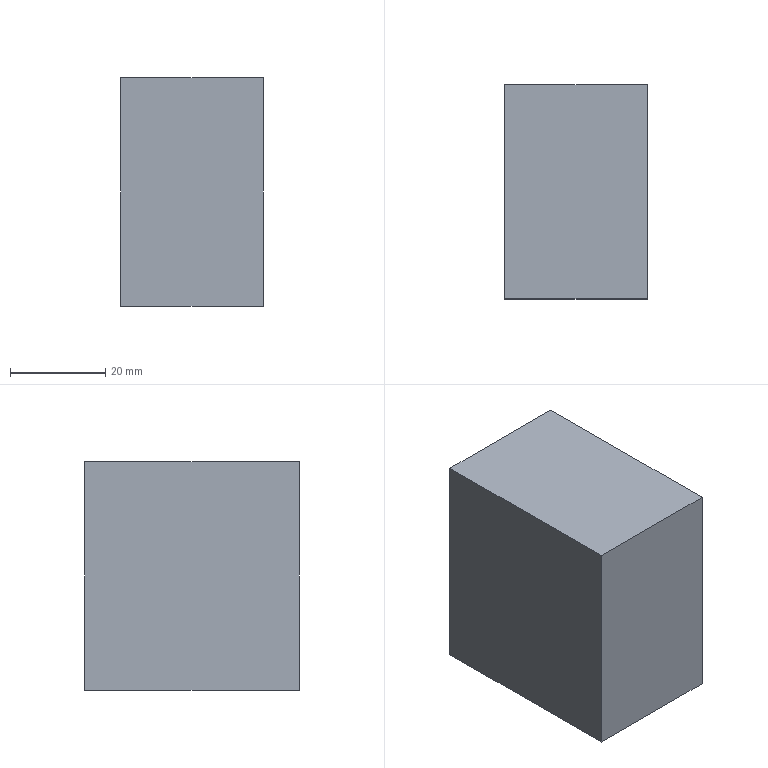Part | STEP file | 1 solid | 14 faces | box 30 x 45 x 48 mm | volume 61923 mm3 | plane 6 | cylinder 4 | cone 4 | commonest cylinder face diameters 8.5 x4
STEP:
#1=CARTESIAN_POINT('',(0.,0.,0.));
#2=DIRECTION('',(0.,0.,1.));
#3=DIRECTION('',(1.,0.,0.));
#4=AXIS2_PLACEMENT_3D('',#1,#2,#3);
#5=CARTESIAN_POINT('',(0.,20.5,-10.75));
#6=VERTEX_POINT('',#5);
#7=CARTESIAN_POINT('',(0.,45.,-10.75));
#8=VERTEX_POINT('',#7);
#9=CARTESIAN_POINT('',(0.,45.,-10.75));
#10=DIRECTION('',(0.,1.,0.));
#11=VECTOR('',#10,1.);
#12=LINE('',#9,#11);
#13=CARTESIAN_POINT('',(0.,45.,-15.));
#14=DIRECTION('',(0.,1.,0.));
#15=DIRECTION('',(0.,0.,1.));
#16=AXIS2_PLACEMENT_3D('',#13,#14,#15);
#17=CYLINDRICAL_SURFACE('',#16,4.25);
#18=CARTESIAN_POINT('',(6.283,0.));
#19=DIRECTION('',(0.,1.));
#20=VECTOR('',#19,1.);
#21=LINE('',#18,#20);
#22=(GEOMETRIC_REPRESENTATION_CONTEXT(2)PARAMETRIC_REPRESENTATION_CONTEXT()REPRESENTATION_CONTEXT('',''));
#23=DEFINITIONAL_REPRESENTATION('',(#21),#22);
#24=PCURVE('',#17,#23);
#25=CARTESIAN_POINT('',(0.,45.,-15.));
#26=DIRECTION('',(0.,1.,0.));
#27=DIRECTION('',(0.,0.,1.));
#28=AXIS2_PLACEMENT_3D('',#25,#26,#27);
#29=CYLINDRICAL_SURFACE('',#28,4.25);
#30=CARTESIAN_POINT('',(0.,0.));
#31=DIRECTION('',(0.,1.));
#32=VECTOR('',#31,1.);
#33=LINE('',#30,#32);
#34=(GEOMETRIC_REPRESENTATION_CONTEXT(2)PARAMETRIC_REPRESENTATION_CONTEXT()REPRESENTATION_CONTEXT('',''));
#35=DEFINITIONAL_REPRESENTATION('',(#33),#34);
#36=PCURVE('',#29,#35);
#37=SURFACE_CURVE('',#12,(#24,#36),.PCURVE_S1.);
#38=EDGE_CURVE('',#6,#8,#37,.T.);
#39=ORIENTED_EDGE('',*,*,#38,.T.);
#40=CARTESIAN_POINT('',(0.,45.,-19.25));
#41=VERTEX_POINT('',#40);
#42=CARTESIAN_POINT('',(0.,45.,-15.));
#43=DIRECTION('',(0.,1.,0.));
#44=DIRECTION('',(0.,0.,1.));
#45=AXIS2_PLACEMENT_3D('',#42,#43,#44);
#46=CIRCLE('',#45,4.25);
#47=CARTESIAN_POINT('',(0.,0.));
#48=DIRECTION('',(1.,0.));
#49=VECTOR('',#48,1.);
#50=LINE('',#47,#49);
#51=(GEOMETRIC_REPRESENTATION_CONTEXT(2)PARAMETRIC_REPRESENTATION_CONTEXT()REPRESENTATION_CONTEXT('',''));
#52=DEFINITIONAL_REPRESENTATION('',(#50),#51);
#53=PCURVE('',#17,#52);
#54=CARTESIAN_POINT('',(0.,45.,0.));
#55=DIRECTION('',(0.,1.,0.));
#56=DIRECTION('',(0.,0.,1.));
#57=AXIS2_PLACEMENT_3D('',#54,#55,#56);
#58=PLANE('',#57);
#59=CARTESIAN_POINT('',(-15.,0.));
#60=DIRECTION('',(1.,0.));
#61=AXIS2_PLACEMENT_2D('',#59,#60);
#62=CIRCLE('',#61,4.25);
#63=(GEOMETRIC_REPRESENTATION_CONTEXT(2)PARAMETRIC_REPRESENTATION_CONTEXT()REPRESENTATION_CONTEXT('',''));
#64=DEFINITIONAL_REPRESENTATION('',(#62),#63);
#65=PCURVE('',#58,#64);
#66=SURFACE_CURVE('',#46,(#53,#65),.PCURVE_S1.);
#67=EDGE_CURVE('',#41,#8,#66,.T.);
#68=ORIENTED_EDGE('',*,*,#67,.F.);
#69=CARTESIAN_POINT('',(0.,20.5,-19.25));
#70=VERTEX_POINT('',#69);
#71=CARTESIAN_POINT('',(0.,45.,-19.25));
#72=DIRECTION('',(0.,1.,0.));
#73=VECTOR('',#72,1.);
#74=LINE('',#71,#73);
#75=CARTESIAN_POINT('',(3.142,0.));
#76=DIRECTION('',(0.,1.));
#77=VECTOR('',#76,1.);
#78=LINE('',#75,#77);
#79=(GEOMETRIC_REPRESENTATION_CONTEXT(2)PARAMETRIC_REPRESENTATION_CONTEXT()REPRESENTATION_CONTEXT('',''));
#80=DEFINITIONAL_REPRESENTATION('',(#78),#79);
#81=PCURVE('',#17,#80);
#82=CARTESIAN_POINT('',(3.142,0.));
#83=DIRECTION('',(0.,1.));
#84=VECTOR('',#83,1.);
#85=LINE('',#82,#84);
#86=(GEOMETRIC_REPRESENTATION_CONTEXT(2)PARAMETRIC_REPRESENTATION_CONTEXT()REPRESENTATION_CONTEXT('',''));
#87=DEFINITIONAL_REPRESENTATION('',(#85),#86);
#88=PCURVE('',#29,#87);
#89=SURFACE_CURVE('',#74,(#81,#88),.PCURVE_S1.);
#90=EDGE_CURVE('',#70,#41,#89,.T.);
#91=ORIENTED_EDGE('',*,*,#90,.F.);
#92=CARTESIAN_POINT('',(0.,20.5,-15.));
#93=DIRECTION('',(0.,1.,0.));
#94=DIRECTION('',(0.,0.,1.));
#95=AXIS2_PLACEMENT_3D('',#92,#93,#94);
#96=CIRCLE('',#95,4.25);
#97=CARTESIAN_POINT('',(0.,-24.5));
#98=DIRECTION('',(1.,0.));
#99=VECTOR('',#98,1.);
#100=LINE('',#97,#99);
#101=(GEOMETRIC_REPRESENTATION_CONTEXT(2)PARAMETRIC_REPRESENTATION_CONTEXT()REPRESENTATION_CONTEXT('',''));
#102=DEFINITIONAL_REPRESENTATION('',(#100),#101);
#103=PCURVE('',#17,#102);
#104=CARTESIAN_POINT('',(0.,20.5,-15.));
#105=DIRECTION('',(0.,1.,0.));
#106=DIRECTION('',(0.,0.,1.));
#107=AXIS2_PLACEMENT_3D('',#104,#105,#106);
#108=CONICAL_SURFACE('',#107,4.25,1.03);
#109=CARTESIAN_POINT('',(0.,0.));
#110=DIRECTION('',(1.,0.));
#111=VECTOR('',#110,1.);
#112=LINE('',#109,#111);
#113=(GEOMETRIC_REPRESENTATION_CONTEXT(2)PARAMETRIC_REPRESENTATION_CONTEXT()REPRESENTATION_CONTEXT('',''));
#114=DEFINITIONAL_REPRESENTATION('',(#112),#113);
#115=PCURVE('',#108,#114);
#116=SURFACE_CURVE('',#96,(#103,#115),.PCURVE_S1.);
#117=EDGE_CURVE('',#70,#6,#116,.T.);
#118=ORIENTED_EDGE('',*,*,#117,.T.);
#119=EDGE_LOOP('',(#39,#68,#91,#118));
#120=FACE_BOUND('',#119,.F.);
#121=ADVANCED_FACE('',(#120),#17,.F.);
#122=ORIENTED_EDGE('',*,*,#117,.F.);
#123=CARTESIAN_POINT('',(0.,17.946,-15.));
#124=VERTEX_POINT('',#123);
#125=CARTESIAN_POINT('',(0.,20.5,-19.25));
#126=DIRECTION('',(0.,0.515,-0.8572));
#127=VECTOR('',#126,1.);
#128=LINE('',#125,#127);
#129=CARTESIAN_POINT('',(3.142,0.));
#130=DIRECTION('',(0.,1.));
#131=VECTOR('',#130,1.);
#132=LINE('',#129,#131);
#133=(GEOMETRIC_REPRESENTATION_CONTEXT(2)PARAMETRIC_REPRESENTATION_CONTEXT()REPRESENTATION_CONTEXT('',''));
#134=DEFINITIONAL_REPRESENTATION('',(#132),#133);
#135=PCURVE('',#108,#134);
#136=CARTESIAN_POINT('',(0.,20.5,-15.));
#137=DIRECTION('',(0.,1.,0.));
#138=DIRECTION('',(0.,0.,1.));
#139=AXIS2_PLACEMENT_3D('',#136,#137,#138);
#140=CONICAL_SURFACE('',#139,4.25,1.03);
#141=CARTESIAN_POINT('',(3.142,0.));
#142=DIRECTION('',(0.,1.));
#143=VECTOR('',#142,1.);
#144=LINE('',#141,#143);
#145=(GEOMETRIC_REPRESENTATION_CONTEXT(2)PARAMETRIC_REPRESENTATION_CONTEXT()REPRESENTATION_CONTEXT('',''));
#146=DEFINITIONAL_REPRESENTATION('',(#144),#145);
#147=PCURVE('',#140,#146);
#148=SURFACE_CURVE('',#128,(#135,#147),.PCURVE_S1.);
#149=EDGE_CURVE('',#124,#70,#148,.T.);
#150=ORIENTED_EDGE('',*,*,#149,.F.);
#151=CARTESIAN_POINT('',(0.,20.5,-10.75));
#152=DIRECTION('',(0.,0.515,0.8572));
#153=VECTOR('',#152,1.);
#154=LINE('',#151,#153);
#155=CARTESIAN_POINT('',(6.283,0.));
#156=DIRECTION('',(0.,1.));
#157=VECTOR('',#156,1.);
#158=LINE('',#155,#157);
#159=(GEOMETRIC_REPRESENTATION_CONTEXT(2)PARAMETRIC_REPRESENTATION_CONTEXT()REPRESENTATION_CONTEXT('',''));
#160=DEFINITIONAL_REPRESENTATION('',(#158),#159);
#161=PCURVE('',#108,#160);
#162=CARTESIAN_POINT('',(0.,0.));
#163=DIRECTION('',(0.,1.));
#164=VECTOR('',#163,1.);
#165=LINE('',#162,#164);
#166=(GEOMETRIC_REPRESENTATION_CONTEXT(2)PARAMETRIC_REPRESENTATION_CONTEXT()REPRESENTATION_CONTEXT('',''));
#167=DEFINITIONAL_REPRESENTATION('',(#165),#166);
#168=PCURVE('',#140,#167);
#169=SURFACE_CURVE('',#154,(#161,#168),.PCURVE_S1.);
#170=EDGE_CURVE('',#124,#6,#169,.T.);
#171=ORIENTED_EDGE('',*,*,#170,.T.);
#172=EDGE_LOOP('',(#122,#150,#171));
#173=FACE_BOUND('',#172,.F.);
#174=ADVANCED_FACE('',(#173),#108,.F.);
#175=CARTESIAN_POINT('',(0.,20.5,19.25));
#176=VERTEX_POINT('',#175);
#177=CARTESIAN_POINT('',(0.,45.,19.25));
#178=VERTEX_POINT('',#177);
#179=CARTESIAN_POINT('',(0.,45.,19.25));
#180=DIRECTION('',(0.,1.,0.));
#181=VECTOR('',#180,1.);
#182=LINE('',#179,#181);
#183=CARTESIAN_POINT('',(0.,45.,15.));
#184=DIRECTION('',(0.,1.,0.));
#185=DIRECTION('',(0.,0.,1.));
#186=AXIS2_PLACEMENT_3D('',#183,#184,#185);
#187=CYLINDRICAL_SURFACE('',#186,4.25);
#188=CARTESIAN_POINT('',(6.283,0.));
#189=DIRECTION('',(0.,1.));
#190=VECTOR('',#189,1.);
#191=LINE('',#188,#190);
#192=(GEOMETRIC_REPRESENTATION_CONTEXT(2)PARAMETRIC_REPRESENTATION_CONTEXT()REPRESENTATION_CONTEXT('',''));
#193=DEFINITIONAL_REPRESENTATION('',(#191),#192);
#194=PCURVE('',#187,#193);
#195=CARTESIAN_POINT('',(0.,45.,15.));
#196=DIRECTION('',(0.,1.,0.));
#197=DIRECTION('',(0.,0.,1.));
#198=AXIS2_PLACEMENT_3D('',#195,#196,#197);
#199=CYLINDRICAL_SURFACE('',#198,4.25);
#200=CARTESIAN_POINT('',(0.,0.));
#201=DIRECTION('',(0.,1.));
#202=VECTOR('',#201,1.);
#203=LINE('',#200,#202);
#204=(GEOMETRIC_REPRESENTATION_CONTEXT(2)PARAMETRIC_REPRESENTATION_CONTEXT()REPRESENTATION_CONTEXT('',''));
#205=DEFINITIONAL_REPRESENTATION('',(#203),#204);
#206=PCURVE('',#199,#205);
#207=SURFACE_CURVE('',#182,(#194,#206),.PCURVE_S1.);
#208=EDGE_CURVE('',#176,#178,#207,.T.);
#209=ORIENTED_EDGE('',*,*,#208,.T.);
#210=CARTESIAN_POINT('',(0.,45.,10.75));
#211=VERTEX_POINT('',#210);
#212=CARTESIAN_POINT('',(0.,45.,15.));
#213=DIRECTION('',(0.,1.,0.));
#214=DIRECTION('',(0.,0.,1.));
#215=AXIS2_PLACEMENT_3D('',#212,#213,#214);
#216=CIRCLE('',#215,4.25);
#217=CARTESIAN_POINT('',(0.,0.));
#218=DIRECTION('',(1.,0.));
#219=VECTOR('',#218,1.);
#220=LINE('',#217,#219);
#221=(GEOMETRIC_REPRESENTATION_CONTEXT(2)PARAMETRIC_REPRESENTATION_CONTEXT()REPRESENTATION_CONTEXT('',''));
#222=DEFINITIONAL_REPRESENTATION('',(#220),#221);
#223=PCURVE('',#187,#222);
#224=CARTESIAN_POINT('',(15.,0.));
#225=DIRECTION('',(1.,0.));
#226=AXIS2_PLACEMENT_2D('',#224,#225);
#227=CIRCLE('',#226,4.25);
#228=(GEOMETRIC_REPRESENTATION_CONTEXT(2)PARAMETRIC_REPRESENTATION_CONTEXT()REPRESENTATION_CONTEXT('',''));
#229=DEFINITIONAL_REPRESENTATION('',(#227),#228);
#230=PCURVE('',#58,#229);
#231=SURFACE_CURVE('',#216,(#223,#230),.PCURVE_S1.);
#232=EDGE_CURVE('',#211,#178,#231,.T.);
#233=ORIENTED_EDGE('',*,*,#232,.F.);
#234=CARTESIAN_POINT('',(0.,20.5,10.75));
#235=VERTEX_POINT('',#234);
#236=CARTESIAN_POINT('',(0.,45.,10.75));
#237=DIRECTION('',(0.,1.,0.));
#238=VECTOR('',#237,1.);
#239=LINE('',#236,#238);
#240=CARTESIAN_POINT('',(3.142,0.));
#241=DIRECTION('',(0.,1.));
#242=VECTOR('',#241,1.);
#243=LINE('',#240,#242);
#244=(GEOMETRIC_REPRESENTATION_CONTEXT(2)PARAMETRIC_REPRESENTATION_CONTEXT()REPRESENTATION_CONTEXT('',''));
#245=DEFINITIONAL_REPRESENTATION('',(#243),#244);
#246=PCURVE('',#187,#245);
#247=CARTESIAN_POINT('',(3.142,0.));
#248=DIRECTION('',(0.,1.));
#249=VECTOR('',#248,1.);
#250=LINE('',#247,#249);
#251=(GEOMETRIC_REPRESENTATION_CONTEXT(2)PARAMETRIC_REPRESENTATION_CONTEXT()REPRESENTATION_CONTEXT('',''));
#252=DEFINITIONAL_REPRESENTATION('',(#250),#251);
#253=PCURVE('',#199,#252);
#254=SURFACE_CURVE('',#239,(#246,#253),.PCURVE_S1.);
#255=EDGE_CURVE('',#235,#211,#254,.T.);
#256=ORIENTED_EDGE('',*,*,#255,.F.);
#257=CARTESIAN_POINT('',(0.,20.5,15.));
#258=DIRECTION('',(0.,1.,0.));
#259=DIRECTION('',(0.,0.,1.));
#260=AXIS2_PLACEMENT_3D('',#257,#258,#259);
#261=CIRCLE('',#260,4.25);
#262=CARTESIAN_POINT('',(0.,-24.5));
#263=DIRECTION('',(1.,0.));
#264=VECTOR('',#263,1.);
#265=LINE('',#262,#264);
#266=(GEOMETRIC_REPRESENTATION_CONTEXT(2)PARAMETRIC_REPRESENTATION_CONTEXT()REPRESENTATION_CONTEXT('',''));
#267=DEFINITIONAL_REPRESENTATION('',(#265),#266);
#268=PCURVE('',#187,#267);
#269=CARTESIAN_POINT('',(0.,20.5,15.));
#270=DIRECTION('',(0.,1.,0.));
#271=DIRECTION('',(0.,0.,1.));
#272=AXIS2_PLACEMENT_3D('',#269,#270,#271);
#273=CONICAL_SURFACE('',#272,4.25,1.03);
#274=CARTESIAN_POINT('',(0.,0.));
#275=DIRECTION('',(1.,0.));
#276=VECTOR('',#275,1.);
#277=LINE('',#274,#276);
#278=(GEOMETRIC_REPRESENTATION_CONTEXT(2)PARAMETRIC_REPRESENTATION_CONTEXT()REPRESENTATION_CONTEXT('',''));
#279=DEFINITIONAL_REPRESENTATION('',(#277),#278);
#280=PCURVE('',#273,#279);
#281=SURFACE_CURVE('',#261,(#268,#280),.PCURVE_S1.);
#282=EDGE_CURVE('',#235,#176,#281,.T.);
#283=ORIENTED_EDGE('',*,*,#282,.T.);
#284=EDGE_LOOP('',(#209,#233,#256,#283));
#285=FACE_BOUND('',#284,.F.);
#286=ADVANCED_FACE('',(#285),#187,.F.);
#287=ORIENTED_EDGE('',*,*,#282,.F.);
#288=CARTESIAN_POINT('',(0.,17.946,15.));
#289=VERTEX_POINT('',#288);
#290=CARTESIAN_POINT('',(0.,20.5,10.75));
#291=DIRECTION('',(0.,0.515,-0.8572));
#292=VECTOR('',#291,1.);
#293=LINE('',#290,#292);
#294=CARTESIAN_POINT('',(3.142,0.));
#295=DIRECTION('',(0.,1.));
#296=VECTOR('',#295,1.);
#297=LINE('',#294,#296);
#298=(GEOMETRIC_REPRESENTATION_CONTEXT(2)PARAMETRIC_REPRESENTATION_CONTEXT()REPRESENTATION_CONTEXT('',''));
#299=DEFINITIONAL_REPRESENTATION('',(#297),#298);
#300=PCURVE('',#273,#299);
#301=CARTESIAN_POINT('',(0.,20.5,15.));
#302=DIRECTION('',(0.,1.,0.));
#303=DIRECTION('',(0.,0.,1.));
#304=AXIS2_PLACEMENT_3D('',#301,#302,#303);
#305=CONICAL_SURFACE('',#304,4.25,1.03);
#306=CARTESIAN_POINT('',(3.142,0.));
#307=DIRECTION('',(0.,1.));
#308=VECTOR('',#307,1.);
#309=LINE('',#306,#308);
#310=(GEOMETRIC_REPRESENTATION_CONTEXT(2)PARAMETRIC_REPRESENTATION_CONTEXT()REPRESENTATION_CONTEXT('',''));
#311=DEFINITIONAL_REPRESENTATION('',(#309),#310);
#312=PCURVE('',#305,#311);
#313=SURFACE_CURVE('',#293,(#300,#312),.PCURVE_S1.);
#314=EDGE_CURVE('',#289,#235,#313,.T.);
#315=ORIENTED_EDGE('',*,*,#314,.F.);
#316=CARTESIAN_POINT('',(0.,20.5,19.25));
#317=DIRECTION('',(0.,0.515,0.8572));
#318=VECTOR('',#317,1.);
#319=LINE('',#316,#318);
#320=CARTESIAN_POINT('',(6.283,0.));
#321=DIRECTION('',(0.,1.));
#322=VECTOR('',#321,1.);
#323=LINE('',#320,#322);
#324=(GEOMETRIC_REPRESENTATION_CONTEXT(2)PARAMETRIC_REPRESENTATION_CONTEXT()REPRESENTATION_CONTEXT('',''));
#325=DEFINITIONAL_REPRESENTATION('',(#323),#324);
#326=PCURVE('',#273,#325);
#327=CARTESIAN_POINT('',(0.,0.));
#328=DIRECTION('',(0.,1.));
#329=VECTOR('',#328,1.);
#330=LINE('',#327,#329);
#331=(GEOMETRIC_REPRESENTATION_CONTEXT(2)PARAMETRIC_REPRESENTATION_CONTEXT()REPRESENTATION_CONTEXT('',''));
#332=DEFINITIONAL_REPRESENTATION('',(#330),#331);
#333=PCURVE('',#305,#332);
#334=SURFACE_CURVE('',#319,(#326,#333),.PCURVE_S1.);
#335=EDGE_CURVE('',#289,#176,#334,.T.);
#336=ORIENTED_EDGE('',*,*,#335,.T.);
#337=EDGE_LOOP('',(#287,#315,#336));
#338=FACE_BOUND('',#337,.F.);
#339=ADVANCED_FACE('',(#338),#273,.F.);
#340=CARTESIAN_POINT('',(-15.,0.,-24.));
#341=VERTEX_POINT('',#340);
#342=CARTESIAN_POINT('',(-15.,0.,24.));
#343=VERTEX_POINT('',#342);
#344=CARTESIAN_POINT('',(-15.,0.,24.));
#345=DIRECTION('',(0.,0.,1.));
#346=VECTOR('',#345,1.);
#347=LINE('',#344,#346);
#348=CARTESIAN_POINT('',(-15.,45.,24.));
#349=DIRECTION('',(1.,0.,0.));
#350=DIRECTION('',(0.,0.,-1.));
#351=AXIS2_PLACEMENT_3D('',#348,#349,#350);
#352=PLANE('',#351);
#353=CARTESIAN_POINT('',(0.,-45.));
#354=DIRECTION('',(-1.,0.));
#355=VECTOR('',#354,1.);
#356=LINE('',#353,#355);
#357=(GEOMETRIC_REPRESENTATION_CONTEXT(2)PARAMETRIC_REPRESENTATION_CONTEXT()REPRESENTATION_CONTEXT('',''));
#358=DEFINITIONAL_REPRESENTATION('',(#356),#357);
#359=PCURVE('',#352,#358);
#360=CARTESIAN_POINT('',(0.,0.,0.));
#361=DIRECTION('',(0.,1.,0.));
#362=DIRECTION('',(0.,0.,1.));
#363=AXIS2_PLACEMENT_3D('',#360,#361,#362);
#364=PLANE('',#363);
#365=CARTESIAN_POINT('',(24.,-15.));
#366=DIRECTION('',(1.,0.));
#367=VECTOR('',#366,1.);
#368=LINE('',#365,#367);
#369=(GEOMETRIC_REPRESENTATION_CONTEXT(2)PARAMETRIC_REPRESENTATION_CONTEXT()REPRESENTATION_CONTEXT('',''));
#370=DEFINITIONAL_REPRESENTATION('',(#368),#369);
#371=PCURVE('',#364,#370);
#372=SURFACE_CURVE('',#347,(#359,#371),.PCURVE_S1.);
#373=EDGE_CURVE('',#341,#343,#372,.T.);
#374=ORIENTED_EDGE('',*,*,#373,.T.);
#375=CARTESIAN_POINT('',(-15.,45.,24.));
#376=VERTEX_POINT('',#375);
#377=CARTESIAN_POINT('',(-15.,45.,24.));
#378=DIRECTION('',(0.,-1.,0.));
#379=VECTOR('',#378,1.);
#380=LINE('',#377,#379);
#381=CARTESIAN_POINT('',(0.,0.));
#382=DIRECTION('',(0.,-1.));
#383=VECTOR('',#382,1.);
#384=LINE('',#381,#383);
#385=(GEOMETRIC_REPRESENTATION_CONTEXT(2)PARAMETRIC_REPRESENTATION_CONTEXT()REPRESENTATION_CONTEXT('',''));
#386=DEFINITIONAL_REPRESENTATION('',(#384),#385);
#387=PCURVE('',#352,#386);
#388=CARTESIAN_POINT('',(15.,45.,24.));
#389=DIRECTION('',(0.,0.,-1.));
#390=DIRECTION('',(-1.,0.,0.));
#391=AXIS2_PLACEMENT_3D('',#388,#389,#390);
#392=PLANE('',#391);
#393=CARTESIAN_POINT('',(30.,0.));
#394=DIRECTION('',(0.,-1.));
#395=VECTOR('',#394,1.);
#396=LINE('',#393,#395);
#397=(GEOMETRIC_REPRESENTATION_CONTEXT(2)PARAMETRIC_REPRESENTATION_CONTEXT()REPRESENTATION_CONTEXT('',''));
#398=DEFINITIONAL_REPRESENTATION('',(#396),#397);
#399=PCURVE('',#392,#398);
#400=SURFACE_CURVE('',#380,(#387,#399),.PCURVE_S1.);
#401=EDGE_CURVE('',#376,#343,#400,.T.);
#402=ORIENTED_EDGE('',*,*,#401,.F.);
#403=CARTESIAN_POINT('',(-15.,45.,-24.));
#404=VERTEX_POINT('',#403);
#405=CARTESIAN_POINT('',(-15.,45.,24.));
#406=DIRECTION('',(0.,0.,1.));
#407=VECTOR('',#406,1.);
#408=LINE('',#405,#407);
#409=CARTESIAN_POINT('',(0.,0.));
#410=DIRECTION('',(-1.,0.));
#411=VECTOR('',#410,1.);
#412=LINE('',#409,#411);
#413=(GEOMETRIC_REPRESENTATION_CONTEXT(2)PARAMETRIC_REPRESENTATION_CONTEXT()REPRESENTATION_CONTEXT('',''));
#414=DEFINITIONAL_REPRESENTATION('',(#412),#413);
#415=PCURVE('',#352,#414);
#416=CARTESIAN_POINT('',(24.,-15.));
#417=DIRECTION('',(1.,0.));
#418=VECTOR('',#417,1.);
#419=LINE('',#416,#418);
#420=(GEOMETRIC_REPRESENTATION_CONTEXT(2)PARAMETRIC_REPRESENTATION_CONTEXT()REPRESENTATION_CONTEXT('',''));
#421=DEFINITIONAL_REPRESENTATION('',(#419),#420);
#422=PCURVE('',#58,#421);
#423=SURFACE_CURVE('',#408,(#415,#422),.PCURVE_S1.);
#424=EDGE_CURVE('',#404,#376,#423,.T.);
#425=ORIENTED_EDGE('',*,*,#424,.F.);
#426=CARTESIAN_POINT('',(-15.,45.,-24.));
#427=DIRECTION('',(0.,-1.,0.));
#428=VECTOR('',#427,1.);
#429=LINE('',#426,#428);
#430=CARTESIAN_POINT('',(48.,0.));
#431=DIRECTION('',(0.,-1.));
#432=VECTOR('',#431,1.);
#433=LINE('',#430,#432);
#434=(GEOMETRIC_REPRESENTATION_CONTEXT(2)PARAMETRIC_REPRESENTATION_CONTEXT()REPRESENTATION_CONTEXT('',''));
#435=DEFINITIONAL_REPRESENTATION('',(#433),#434);
#436=PCURVE('',#352,#435);
#437=CARTESIAN_POINT('',(15.,45.,-24.));
#438=DIRECTION('',(0.,0.,1.));
#439=DIRECTION('',(1.,0.,0.));
#440=AXIS2_PLACEMENT_3D('',#437,#438,#439);
#441=PLANE('',#440);
#442=CARTESIAN_POINT('',(-30.,0.));
#443=DIRECTION('',(0.,-1.));
#444=VECTOR('',#443,1.);
#445=LINE('',#442,#444);
#446=(GEOMETRIC_REPRESENTATION_CONTEXT(2)PARAMETRIC_REPRESENTATION_CONTEXT()REPRESENTATION_CONTEXT('',''));
#447=DEFINITIONAL_REPRESENTATION('',(#445),#446);
#448=PCURVE('',#441,#447);
#449=SURFACE_CURVE('',#429,(#436,#448),.PCURVE_S1.);
#450=EDGE_CURVE('',#404,#341,#449,.T.);
#451=ORIENTED_EDGE('',*,*,#450,.T.);
#452=EDGE_LOOP('',(#374,#402,#425,#451));
#453=FACE_BOUND('',#452,.T.);
#454=ADVANCED_FACE('',(#453),#352,.F.);
#455=CARTESIAN_POINT('',(15.,0.,24.));
#456=VERTEX_POINT('',#455);
#457=CARTESIAN_POINT('',(15.,0.,24.));
#458=DIRECTION('',(1.,0.,0.));
#459=VECTOR('',#458,1.);
#460=LINE('',#457,#459);
#461=CARTESIAN_POINT('',(0.,-45.));
#462=DIRECTION('',(-1.,0.));
#463=VECTOR('',#462,1.);
#464=LINE('',#461,#463);
#465=(GEOMETRIC_REPRESENTATION_CONTEXT(2)PARAMETRIC_REPRESENTATION_CONTEXT()REPRESENTATION_CONTEXT('',''));
#466=DEFINITIONAL_REPRESENTATION('',(#464),#465);
#467=PCURVE('',#392,#466);
#468=CARTESIAN_POINT('',(24.,15.));
#469=DIRECTION('',(0.,1.));
#470=VECTOR('',#469,1.);
#471=LINE('',#468,#470);
#472=(GEOMETRIC_REPRESENTATION_CONTEXT(2)PARAMETRIC_REPRESENTATION_CONTEXT()REPRESENTATION_CONTEXT('',''));
#473=DEFINITIONAL_REPRESENTATION('',(#471),#472);
#474=PCURVE('',#364,#473);
#475=SURFACE_CURVE('',#460,(#467,#474),.PCURVE_S1.);
#476=EDGE_CURVE('',#343,#456,#475,.T.);
#477=ORIENTED_EDGE('',*,*,#476,.T.);
#478=CARTESIAN_POINT('',(15.,45.,24.));
#479=VERTEX_POINT('',#478);
#480=CARTESIAN_POINT('',(15.,45.,24.));
#481=DIRECTION('',(0.,-1.,0.));
#482=VECTOR('',#481,1.);
#483=LINE('',#480,#482);
#484=CARTESIAN_POINT('',(0.,0.));
#485=DIRECTION('',(0.,-1.));
#486=VECTOR('',#485,1.);
#487=LINE('',#484,#486);
#488=(GEOMETRIC_REPRESENTATION_CONTEXT(2)PARAMETRIC_REPRESENTATION_CONTEXT()REPRESENTATION_CONTEXT('',''));
#489=DEFINITIONAL_REPRESENTATION('',(#487),#488);
#490=PCURVE('',#392,#489);
#491=CARTESIAN_POINT('',(15.,45.,24.));
#492=DIRECTION('',(-1.,0.,0.));
#493=DIRECTION('',(0.,0.,1.));
#494=AXIS2_PLACEMENT_3D('',#491,#492,#493);
#495=PLANE('',#494);
#496=CARTESIAN_POINT('',(0.,0.));
#497=DIRECTION('',(0.,-1.));
#498=VECTOR('',#497,1.);
#499=LINE('',#496,#498);
#500=(GEOMETRIC_REPRESENTATION_CONTEXT(2)PARAMETRIC_REPRESENTATION_CONTEXT()REPRESENTATION_CONTEXT('',''));
#501=DEFINITIONAL_REPRESENTATION('',(#499),#500);
#502=PCURVE('',#495,#501);
#503=SURFACE_CURVE('',#483,(#490,#502),.PCURVE_S1.);
#504=EDGE_CURVE('',#479,#456,#503,.T.);
#505=ORIENTED_EDGE('',*,*,#504,.F.);
#506=CARTESIAN_POINT('',(15.,45.,24.));
#507=DIRECTION('',(1.,0.,0.));
#508=VECTOR('',#507,1.);
#509=LINE('',#506,#508);
#510=CARTESIAN_POINT('',(0.,0.));
#511=DIRECTION('',(-1.,0.));
#512=VECTOR('',#511,1.);
#513=LINE('',#510,#512);
#514=(GEOMETRIC_REPRESENTATION_CONTEXT(2)PARAMETRIC_REPRESENTATION_CONTEXT()REPRESENTATION_CONTEXT('',''));
#515=DEFINITIONAL_REPRESENTATION('',(#513),#514);
#516=PCURVE('',#392,#515);
#517=CARTESIAN_POINT('',(24.,15.));
#518=DIRECTION('',(0.,1.));
#519=VECTOR('',#518,1.);
#520=LINE('',#517,#519);
#521=(GEOMETRIC_REPRESENTATION_CONTEXT(2)PARAMETRIC_REPRESENTATION_CONTEXT()REPRESENTATION_CONTEXT('',''));
#522=DEFINITIONAL_REPRESENTATION('',(#520),#521);
#523=PCURVE('',#58,#522);
#524=SURFACE_CURVE('',#509,(#516,#523),.PCURVE_S1.);
#525=EDGE_CURVE('',#376,#479,#524,.T.);
#526=ORIENTED_EDGE('',*,*,#525,.F.);
#527=ORIENTED_EDGE('',*,*,#401,.T.);
#528=EDGE_LOOP('',(#477,#505,#526,#527));
#529=FACE_BOUND('',#528,.T.);
#530=ADVANCED_FACE('',(#529),#392,.F.);
#531=CARTESIAN_POINT('',(15.,0.,-24.));
#532=VERTEX_POINT('',#531);
#533=CARTESIAN_POINT('',(15.,0.,24.));
#534=DIRECTION('',(0.,0.,-1.));
#535=VECTOR('',#534,1.);
#536=LINE('',#533,#535);
#537=CARTESIAN_POINT('',(0.,-45.));
#538=DIRECTION('',(-1.,0.));
#539=VECTOR('',#538,1.);
#540=LINE('',#537,#539);
#541=(GEOMETRIC_REPRESENTATION_CONTEXT(2)PARAMETRIC_REPRESENTATION_CONTEXT()REPRESENTATION_CONTEXT('',''));
#542=DEFINITIONAL_REPRESENTATION('',(#540),#541);
#543=PCURVE('',#495,#542);
#544=CARTESIAN_POINT('',(24.,15.));
#545=DIRECTION('',(-1.,0.));
#546=VECTOR('',#545,1.);
#547=LINE('',#544,#546);
#548=(GEOMETRIC_REPRESENTATION_CONTEXT(2)PARAMETRIC_REPRESENTATION_CONTEXT()REPRESENTATION_CONTEXT('',''));
#549=DEFINITIONAL_REPRESENTATION('',(#547),#548);
#550=PCURVE('',#364,#549);
#551=SURFACE_CURVE('',#536,(#543,#550),.PCURVE_S1.);
#552=EDGE_CURVE('',#456,#532,#551,.T.);
#553=ORIENTED_EDGE('',*,*,#552,.T.);
#554=CARTESIAN_POINT('',(15.,45.,-24.));
#555=VERTEX_POINT('',#554);
#556=CARTESIAN_POINT('',(15.,45.,-24.));
#557=DIRECTION('',(0.,-1.,0.));
#558=VECTOR('',#557,1.);
#559=LINE('',#556,#558);
#560=CARTESIAN_POINT('',(-48.,0.));
#561=DIRECTION('',(0.,-1.));
#562=VECTOR('',#561,1.);
#563=LINE('',#560,#562);
#564=(GEOMETRIC_REPRESENTATION_CONTEXT(2)PARAMETRIC_REPRESENTATION_CONTEXT()REPRESENTATION_CONTEXT('',''));
#565=DEFINITIONAL_REPRESENTATION('',(#563),#564);
#566=PCURVE('',#495,#565);
#567=CARTESIAN_POINT('',(0.,0.));
#568=DIRECTION('',(0.,-1.));
#569=VECTOR('',#568,1.);
#570=LINE('',#567,#569);
#571=(GEOMETRIC_REPRESENTATION_CONTEXT(2)PARAMETRIC_REPRESENTATION_CONTEXT()REPRESENTATION_CONTEXT('',''));
#572=DEFINITIONAL_REPRESENTATION('',(#570),#571);
#573=PCURVE('',#441,#572);
#574=SURFACE_CURVE('',#559,(#566,#573),.PCURVE_S1.);
#575=EDGE_CURVE('',#555,#532,#574,.T.);
#576=ORIENTED_EDGE('',*,*,#575,.F.);
#577=CARTESIAN_POINT('',(15.,45.,24.));
#578=DIRECTION('',(0.,0.,-1.));
#579=VECTOR('',#578,1.);
#580=LINE('',#577,#579);
#581=CARTESIAN_POINT('',(0.,0.));
#582=DIRECTION('',(-1.,0.));
#583=VECTOR('',#582,1.);
#584=LINE('',#581,#583);
#585=(GEOMETRIC_REPRESENTATION_CONTEXT(2)PARAMETRIC_REPRESENTATION_CONTEXT()REPRESENTATION_CONTEXT('',''));
#586=DEFINITIONAL_REPRESENTATION('',(#584),#585);
#587=PCURVE('',#495,#586);
#588=CARTESIAN_POINT('',(24.,15.));
#589=DIRECTION('',(-1.,0.));
#590=VECTOR('',#589,1.);
#591=LINE('',#588,#590);
#592=(GEOMETRIC_REPRESENTATION_CONTEXT(2)PARAMETRIC_REPRESENTATION_CONTEXT()REPRESENTATION_CONTEXT('',''));
#593=DEFINITIONAL_REPRESENTATION('',(#591),#592);
#594=PCURVE('',#58,#593);
#595=SURFACE_CURVE('',#580,(#587,#594),.PCURVE_S1.);
#596=EDGE_CURVE('',#479,#555,#595,.T.);
#597=ORIENTED_EDGE('',*,*,#596,.F.);
#598=ORIENTED_EDGE('',*,*,#504,.T.);
#599=EDGE_LOOP('',(#553,#576,#597,#598));
#600=FACE_BOUND('',#599,.T.);
#601=ADVANCED_FACE('',(#600),#495,.F.);
#602=CARTESIAN_POINT('',(15.,0.,-24.));
#603=DIRECTION('',(-1.,0.,0.));
#604=VECTOR('',#603,1.);
#605=LINE('',#602,#604);
#606=CARTESIAN_POINT('',(0.,-45.));
#607=DIRECTION('',(-1.,0.));
#608=VECTOR('',#607,1.);
#609=LINE('',#606,#608);
#610=(GEOMETRIC_REPRESENTATION_CONTEXT(2)PARAMETRIC_REPRESENTATION_CONTEXT()REPRESENTATION_CONTEXT('',''));
#611=DEFINITIONAL_REPRESENTATION('',(#609),#610);
#612=PCURVE('',#441,#611);
#613=CARTESIAN_POINT('',(-24.,15.));
#614=DIRECTION('',(0.,-1.));
#615=VECTOR('',#614,1.);
#616=LINE('',#613,#615);
#617=(GEOMETRIC_REPRESENTATION_CONTEXT(2)PARAMETRIC_REPRESENTATION_CONTEXT()REPRESENTATION_CONTEXT('',''));
#618=DEFINITIONAL_REPRESENTATION('',(#616),#617);
#619=PCURVE('',#364,#618);
#620=SURFACE_CURVE('',#605,(#612,#619),.PCURVE_S1.);
#621=EDGE_CURVE('',#532,#341,#620,.T.);
#622=ORIENTED_EDGE('',*,*,#621,.T.);
#623=ORIENTED_EDGE('',*,*,#450,.F.);
#624=CARTESIAN_POINT('',(15.,45.,-24.));
#625=DIRECTION('',(-1.,0.,0.));
#626=VECTOR('',#625,1.);
#627=LINE('',#624,#626);
#628=CARTESIAN_POINT('',(0.,0.));
#629=DIRECTION('',(-1.,0.));
#630=VECTOR('',#629,1.);
#631=LINE('',#628,#630);
#632=(GEOMETRIC_REPRESENTATION_CONTEXT(2)PARAMETRIC_REPRESENTATION_CONTEXT()REPRESENTATION_CONTEXT('',''));
#633=DEFINITIONAL_REPRESENTATION('',(#631),#632);
#634=PCURVE('',#441,#633);
#635=CARTESIAN_POINT('',(-24.,15.));
#636=DIRECTION('',(0.,-1.));
#637=VECTOR('',#636,1.);
#638=LINE('',#635,#637);
#639=(GEOMETRIC_REPRESENTATION_CONTEXT(2)PARAMETRIC_REPRESENTATION_CONTEXT()REPRESENTATION_CONTEXT('',''));
#640=DEFINITIONAL_REPRESENTATION('',(#638),#639);
#641=PCURVE('',#58,#640);
#642=SURFACE_CURVE('',#627,(#634,#641),.PCURVE_S1.);
#643=EDGE_CURVE('',#555,#404,#642,.T.);
#644=ORIENTED_EDGE('',*,*,#643,.F.);
#645=ORIENTED_EDGE('',*,*,#575,.T.);
#646=EDGE_LOOP('',(#622,#623,#644,#645));
#647=FACE_BOUND('',#646,.T.);
#648=ADVANCED_FACE('',(#647),#441,.F.);
#649=CARTESIAN_POINT('',(0.,45.,-15.));
#650=DIRECTION('',(0.,1.,0.));
#651=DIRECTION('',(0.,0.,1.));
#652=AXIS2_PLACEMENT_3D('',#649,#650,#651);
#653=CIRCLE('',#652,4.25);
#654=CARTESIAN_POINT('',(-15.,0.));
#655=DIRECTION('',(1.,0.));
#656=AXIS2_PLACEMENT_2D('',#654,#655);
#657=CIRCLE('',#656,4.25);
#658=(GEOMETRIC_REPRESENTATION_CONTEXT(2)PARAMETRIC_REPRESENTATION_CONTEXT()REPRESENTATION_CONTEXT('',''));
#659=DEFINITIONAL_REPRESENTATION('',(#657),#658);
#660=PCURVE('',#58,#659);
#661=CARTESIAN_POINT('',(0.,0.));
#662=DIRECTION('',(1.,0.));
#663=VECTOR('',#662,1.);
#664=LINE('',#661,#663);
#665=(GEOMETRIC_REPRESENTATION_CONTEXT(2)PARAMETRIC_REPRESENTATION_CONTEXT()REPRESENTATION_CONTEXT('',''));
#666=DEFINITIONAL_REPRESENTATION('',(#664),#665);
#667=PCURVE('',#29,#666);
#668=SURFACE_CURVE('',#653,(#660,#667),.PCURVE_S1.);
#669=EDGE_CURVE('',#8,#41,#668,.T.);
#670=ORIENTED_EDGE('',*,*,#669,.F.);
#671=ORIENTED_EDGE('',*,*,#67,.F.);
#672=EDGE_LOOP('',(#670,#671));
#673=FACE_BOUND('',#672,.T.);
#674=CARTESIAN_POINT('',(0.,45.,15.));
#675=DIRECTION('',(0.,1.,0.));
#676=DIRECTION('',(0.,0.,1.));
#677=AXIS2_PLACEMENT_3D('',#674,#675,#676);
#678=CIRCLE('',#677,4.25);
#679=CARTESIAN_POINT('',(15.,0.));
#680=DIRECTION('',(1.,0.));
#681=AXIS2_PLACEMENT_2D('',#679,#680);
#682=CIRCLE('',#681,4.25);
#683=(GEOMETRIC_REPRESENTATION_CONTEXT(2)PARAMETRIC_REPRESENTATION_CONTEXT()REPRESENTATION_CONTEXT('',''));
#684=DEFINITIONAL_REPRESENTATION('',(#682),#683);
#685=PCURVE('',#58,#684);
#686=CARTESIAN_POINT('',(0.,0.));
#687=DIRECTION('',(1.,0.));
#688=VECTOR('',#687,1.);
#689=LINE('',#686,#688);
#690=(GEOMETRIC_REPRESENTATION_CONTEXT(2)PARAMETRIC_REPRESENTATION_CONTEXT()REPRESENTATION_CONTEXT('',''));
#691=DEFINITIONAL_REPRESENTATION('',(#689),#690);
#692=PCURVE('',#199,#691);
#693=SURFACE_CURVE('',#678,(#685,#692),.PCURVE_S1.);
#694=EDGE_CURVE('',#178,#211,#693,.T.);
#695=ORIENTED_EDGE('',*,*,#694,.F.);
#696=ORIENTED_EDGE('',*,*,#232,.F.);
#697=EDGE_LOOP('',(#695,#696));
#698=FACE_BOUND('',#697,.T.);
#699=ORIENTED_EDGE('',*,*,#424,.T.);
#700=ORIENTED_EDGE('',*,*,#525,.T.);
#701=ORIENTED_EDGE('',*,*,#596,.T.);
#702=ORIENTED_EDGE('',*,*,#643,.T.);
#703=EDGE_LOOP('',(#699,#700,#701,#702));
#704=FACE_BOUND('',#703,.T.);
#705=ADVANCED_FACE('',(#673,#698,#704),#58,.T.);
#706=ORIENTED_EDGE('',*,*,#373,.F.);
#707=ORIENTED_EDGE('',*,*,#621,.F.);
#708=ORIENTED_EDGE('',*,*,#552,.F.);
#709=ORIENTED_EDGE('',*,*,#476,.F.);
#710=EDGE_LOOP('',(#706,#707,#708,#709));
#711=FACE_BOUND('',#710,.T.);
#712=ADVANCED_FACE('',(#711),#364,.F.);
#713=CARTESIAN_POINT('',(0.,20.5,15.));
#714=DIRECTION('',(0.,1.,0.));
#715=DIRECTION('',(0.,0.,1.));
#716=AXIS2_PLACEMENT_3D('',#713,#714,#715);
#717=CIRCLE('',#716,4.25);
#718=CARTESIAN_POINT('',(0.,0.));
#719=DIRECTION('',(1.,0.));
#720=VECTOR('',#719,1.);
#721=LINE('',#718,#720);
#722=(GEOMETRIC_REPRESENTATION_CONTEXT(2)PARAMETRIC_REPRESENTATION_CONTEXT()REPRESENTATION_CONTEXT('',''));
#723=DEFINITIONAL_REPRESENTATION('',(#721),#722);
#724=PCURVE('',#305,#723);
#725=CARTESIAN_POINT('',(0.,-24.5));
#726=DIRECTION('',(1.,0.));
#727=VECTOR('',#726,1.);
#728=LINE('',#725,#727);
#729=(GEOMETRIC_REPRESENTATION_CONTEXT(2)PARAMETRIC_REPRESENTATION_CONTEXT()REPRESENTATION_CONTEXT('',''));
#730=DEFINITIONAL_REPRESENTATION('',(#728),#729);
#731=PCURVE('',#199,#730);
#732=SURFACE_CURVE('',#717,(#724,#731),.PCURVE_S1.);
#733=EDGE_CURVE('',#176,#235,#732,.T.);
#734=ORIENTED_EDGE('',*,*,#733,.F.);
#735=ORIENTED_EDGE('',*,*,#335,.F.);
#736=ORIENTED_EDGE('',*,*,#314,.T.);
#737=EDGE_LOOP('',(#734,#735,#736));
#738=FACE_BOUND('',#737,.F.);
#739=ADVANCED_FACE('',(#738),#305,.F.);
#740=ORIENTED_EDGE('',*,*,#694,.F.);
#741=ORIENTED_EDGE('',*,*,#208,.F.);
#742=ORIENTED_EDGE('',*,*,#733,.T.);
#743=ORIENTED_EDGE('',*,*,#255,.T.);
#744=EDGE_LOOP('',(#740,#741,#742,#743));
#745=FACE_BOUND('',#744,.F.);
#746=ADVANCED_FACE('',(#745),#199,.F.);
#747=CARTESIAN_POINT('',(0.,20.5,-15.));
#748=DIRECTION('',(0.,1.,0.));
#749=DIRECTION('',(0.,0.,1.));
#750=AXIS2_PLACEMENT_3D('',#747,#748,#749);
#751=CIRCLE('',#750,4.25);
#752=CARTESIAN_POINT('',(0.,0.));
#753=DIRECTION('',(1.,0.));
#754=VECTOR('',#753,1.);
#755=LINE('',#752,#754);
#756=(GEOMETRIC_REPRESENTATION_CONTEXT(2)PARAMETRIC_REPRESENTATION_CONTEXT()REPRESENTATION_CONTEXT('',''));
#757=DEFINITIONAL_REPRESENTATION('',(#755),#756);
#758=PCURVE('',#140,#757);
#759=CARTESIAN_POINT('',(0.,-24.5));
#760=DIRECTION('',(1.,0.));
#761=VECTOR('',#760,1.);
#762=LINE('',#759,#761);
#763=(GEOMETRIC_REPRESENTATION_CONTEXT(2)PARAMETRIC_REPRESENTATION_CONTEXT()REPRESENTATION_CONTEXT('',''));
#764=DEFINITIONAL_REPRESENTATION('',(#762),#763);
#765=PCURVE('',#29,#764);
#766=SURFACE_CURVE('',#751,(#758,#765),.PCURVE_S1.);
#767=EDGE_CURVE('',#6,#70,#766,.T.);
#768=ORIENTED_EDGE('',*,*,#767,.F.);
#769=ORIENTED_EDGE('',*,*,#170,.F.);
#770=ORIENTED_EDGE('',*,*,#149,.T.);
#771=EDGE_LOOP('',(#768,#769,#770));
#772=FACE_BOUND('',#771,.F.);
#773=ADVANCED_FACE('',(#772),#140,.F.);
#774=ORIENTED_EDGE('',*,*,#669,.F.);
#775=ORIENTED_EDGE('',*,*,#38,.F.);
#776=ORIENTED_EDGE('',*,*,#767,.T.);
#777=ORIENTED_EDGE('',*,*,#90,.T.);
#778=EDGE_LOOP('',(#774,#775,#776,#777));
#779=FACE_BOUND('',#778,.F.);
#780=ADVANCED_FACE('',(#779),#29,.F.);
#781=CLOSED_SHELL('',(#121,#174,#286,#339,#454,#530,#601,#648,#705,#712,#739,#746,#773,#780));
#782=MANIFOLD_SOLID_BREP('',#781);
#783=(LENGTH_UNIT()NAMED_UNIT(*)SI_UNIT(.MILLI.,.METRE.));
#784=UNCERTAINTY_MEASURE_WITH_UNIT(LENGTH_MEASURE(0.0000001),#783,'','');
#785=(NAMED_UNIT(*)PLANE_ANGLE_UNIT()SI_UNIT($,.RADIAN.));
#786=(NAMED_UNIT(*)SI_UNIT($,.STERADIAN.)SOLID_ANGLE_UNIT());
#787=(GEOMETRIC_REPRESENTATION_CONTEXT(3)GLOBAL_UNCERTAINTY_ASSIGNED_CONTEXT((#784))GLOBAL_UNIT_ASSIGNED_CONTEXT((#783,#785,#786))REPRESENTATION_CONTEXT('',''));
#788=ADVANCED_BREP_SHAPE_REPRESENTATION('',(#4,#782),#787);